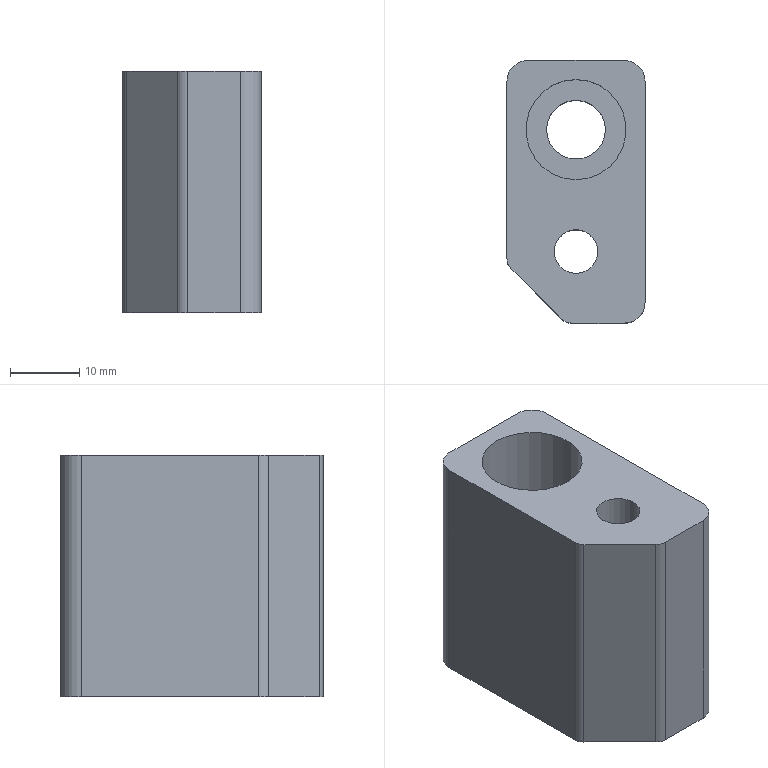Part | NX | features DIE-15 2 | 1 solid | 18 faces | box 20 x 38 x 35 mm | volume 20161 mm3 | plane 9 | cylinder 9 | commonest cylinder face diameters 6 x3 4 x2 6.29 x1 8.29 x1 8.506 x1 14.5 x1
STEP:
#1=CARTESIAN_POINT('',(2411.699,-772.697,858.716));
#2=VERTEX_POINT('',#1);
#3=CARTESIAN_POINT('',(2411.699,-772.697,823.716));
#4=VERTEX_POINT('',#3);
#5=CARTESIAN_POINT('',(2411.699,-772.697,858.716));
#6=DIRECTION('',(0.,0.,-1.));
#7=VECTOR('',#6,1000.);
#8=LINE('',#5,#7);
#9=EDGE_CURVE('',#2,#4,#8,.T.);
#10=ORIENTED_EDGE('',*,*,#9,.F.);
#11=CARTESIAN_POINT('',(2411.699,-804.697,858.716));
#12=VERTEX_POINT('',#11);
#13=CARTESIAN_POINT('',(2411.699,-787.697,858.716));
#14=DIRECTION('',(0.,1.,0.));
#15=VECTOR('',#14,1000.);
#16=LINE('',#13,#15);
#17=EDGE_CURVE('',#12,#2,#16,.T.);
#18=ORIENTED_EDGE('',*,*,#17,.F.);
#19=CARTESIAN_POINT('',(2411.699,-804.697,823.716));
#20=VERTEX_POINT('',#19);
#21=CARTESIAN_POINT('',(2411.699,-804.697,858.716));
#22=DIRECTION('',(0.,0.,-1.));
#23=VECTOR('',#22,1000.);
#24=LINE('',#21,#23);
#25=EDGE_CURVE('',#20,#12,#24,.F.);
#26=ORIENTED_EDGE('',*,*,#25,.F.);
#27=CARTESIAN_POINT('',(2411.699,-787.697,823.716));
#28=DIRECTION('',(0.,-1.,0.));
#29=VECTOR('',#28,1000.);
#30=LINE('',#27,#29);
#31=EDGE_CURVE('',#4,#20,#30,.T.);
#32=ORIENTED_EDGE('',*,*,#31,.F.);
#33=EDGE_LOOP('',(#10,#18,#26,#32));
#34=FACE_BOUND('',#33,.T.);
#35=CARTESIAN_POINT('',(2411.699,-787.697,858.716));
#36=DIRECTION('',(1.,0.,0.));
#37=DIRECTION('',(0.,0.,1.));
#38=AXIS2_PLACEMENT_3D('',#35,#36,#37);
#39=PLANE('',#38);
#40=ADVANCED_FACE('',(#34),#39,.T.);
#41=CARTESIAN_POINT('',(2408.699,-807.697,858.716));
#42=VERTEX_POINT('',#41);
#43=CARTESIAN_POINT('',(2408.699,-807.697,823.716));
#44=VERTEX_POINT('',#43);
#45=CARTESIAN_POINT('',(2408.699,-807.697,858.716));
#46=DIRECTION('',(0.,0.,-1.));
#47=VECTOR('',#46,1000.);
#48=LINE('',#45,#47);
#49=EDGE_CURVE('',#42,#44,#48,.T.);
#50=ORIENTED_EDGE('',*,*,#49,.F.);
#51=CARTESIAN_POINT('',(2401.063,-807.697,858.716));
#52=VERTEX_POINT('',#51);
#53=CARTESIAN_POINT('',(2401.699,-807.697,858.716));
#54=DIRECTION('',(1.,0.,0.));
#55=VECTOR('',#54,1000.);
#56=LINE('',#53,#55);
#57=EDGE_CURVE('',#52,#42,#56,.T.);
#58=ORIENTED_EDGE('',*,*,#57,.F.);
#59=CARTESIAN_POINT('',(2401.063,-807.697,823.716));
#60=VERTEX_POINT('',#59);
#61=CARTESIAN_POINT('',(2401.063,-807.697,858.716));
#62=DIRECTION('',(0.,0.,-1.));
#63=VECTOR('',#62,1000.);
#64=LINE('',#61,#63);
#65=EDGE_CURVE('',#52,#60,#64,.T.);
#66=ORIENTED_EDGE('',*,*,#65,.T.);
#67=CARTESIAN_POINT('',(2401.699,-807.697,823.716));
#68=DIRECTION('',(-1.,0.,0.));
#69=VECTOR('',#68,1000.);
#70=LINE('',#67,#69);
#71=EDGE_CURVE('',#44,#60,#70,.T.);
#72=ORIENTED_EDGE('',*,*,#71,.F.);
#73=EDGE_LOOP('',(#50,#58,#66,#72));
#74=FACE_BOUND('',#73,.T.);
#75=CARTESIAN_POINT('',(2401.699,-807.697,858.716));
#76=DIRECTION('',(0.,-1.,0.));
#77=DIRECTION('',(0.,0.,-1.));
#78=AXIS2_PLACEMENT_3D('',#75,#76,#77);
#79=PLANE('',#78);
#80=ADVANCED_FACE('',(#74),#79,.T.);
#81=CARTESIAN_POINT('',(2391.699,-798.333,823.716));
#82=VERTEX_POINT('',#81);
#83=CARTESIAN_POINT('',(2391.699,-798.333,858.716));
#84=VERTEX_POINT('',#83);
#85=CARTESIAN_POINT('',(2391.699,-798.333,858.716));
#86=DIRECTION('',(0.,0.,1.));
#87=VECTOR('',#86,1000.);
#88=LINE('',#85,#87);
#89=EDGE_CURVE('',#82,#84,#88,.T.);
#90=ORIENTED_EDGE('',*,*,#89,.T.);
#91=CARTESIAN_POINT('',(2391.699,-772.697,858.716));
#92=VERTEX_POINT('',#91);
#93=CARTESIAN_POINT('',(2391.699,-787.697,858.716));
#94=DIRECTION('',(0.,-1.,0.));
#95=VECTOR('',#94,1000.);
#96=LINE('',#93,#95);
#97=EDGE_CURVE('',#92,#84,#96,.T.);
#98=ORIENTED_EDGE('',*,*,#97,.F.);
#99=CARTESIAN_POINT('',(2391.699,-772.697,823.716));
#100=VERTEX_POINT('',#99);
#101=CARTESIAN_POINT('',(2391.699,-772.697,858.716));
#102=DIRECTION('',(0.,0.,-1.));
#103=VECTOR('',#102,1000.);
#104=LINE('',#101,#103);
#105=EDGE_CURVE('',#100,#92,#104,.F.);
#106=ORIENTED_EDGE('',*,*,#105,.F.);
#107=CARTESIAN_POINT('',(2391.699,-787.697,823.716));
#108=DIRECTION('',(0.,1.,0.));
#109=VECTOR('',#108,1000.);
#110=LINE('',#107,#109);
#111=EDGE_CURVE('',#82,#100,#110,.T.);
#112=ORIENTED_EDGE('',*,*,#111,.F.);
#113=EDGE_LOOP('',(#90,#98,#106,#112));
#114=FACE_BOUND('',#113,.T.);
#115=CARTESIAN_POINT('',(2391.699,-787.697,858.716));
#116=DIRECTION('',(-1.,0.,0.));
#117=DIRECTION('',(0.,0.,-1.));
#118=AXIS2_PLACEMENT_3D('',#115,#116,#117);
#119=PLANE('',#118);
#120=ADVANCED_FACE('',(#114),#119,.T.);
#121=CARTESIAN_POINT('',(2394.699,-769.697,858.716));
#122=VERTEX_POINT('',#121);
#123=CARTESIAN_POINT('',(2394.699,-769.697,823.716));
#124=VERTEX_POINT('',#123);
#125=CARTESIAN_POINT('',(2394.699,-769.697,858.716));
#126=DIRECTION('',(0.,0.,-1.));
#127=VECTOR('',#126,1000.);
#128=LINE('',#125,#127);
#129=EDGE_CURVE('',#122,#124,#128,.T.);
#130=ORIENTED_EDGE('',*,*,#129,.F.);
#131=CARTESIAN_POINT('',(2408.699,-769.697,858.716));
#132=VERTEX_POINT('',#131);
#133=CARTESIAN_POINT('',(2401.699,-769.697,858.716));
#134=DIRECTION('',(-1.,0.,0.));
#135=VECTOR('',#134,1000.);
#136=LINE('',#133,#135);
#137=EDGE_CURVE('',#132,#122,#136,.T.);
#138=ORIENTED_EDGE('',*,*,#137,.F.);
#139=CARTESIAN_POINT('',(2408.699,-769.697,823.716));
#140=VERTEX_POINT('',#139);
#141=CARTESIAN_POINT('',(2408.699,-769.697,858.716));
#142=DIRECTION('',(0.,0.,-1.));
#143=VECTOR('',#142,1000.);
#144=LINE('',#141,#143);
#145=EDGE_CURVE('',#140,#132,#144,.F.);
#146=ORIENTED_EDGE('',*,*,#145,.F.);
#147=CARTESIAN_POINT('',(2401.699,-769.697,823.716));
#148=DIRECTION('',(1.,0.,0.));
#149=VECTOR('',#148,1000.);
#150=LINE('',#147,#149);
#151=EDGE_CURVE('',#124,#140,#150,.T.);
#152=ORIENTED_EDGE('',*,*,#151,.F.);
#153=EDGE_LOOP('',(#130,#138,#146,#152));
#154=FACE_BOUND('',#153,.T.);
#155=CARTESIAN_POINT('',(2401.699,-769.697,858.716));
#156=DIRECTION('',(0.,1.,0.));
#157=DIRECTION('',(0.,0.,1.));
#158=AXIS2_PLACEMENT_3D('',#155,#156,#157);
#159=PLANE('',#158);
#160=ADVANCED_FACE('',(#154),#159,.T.);
#161=CARTESIAN_POINT('',(2399.649,-807.111,823.716));
#162=VERTEX_POINT('',#161);
#163=CARTESIAN_POINT('',(2399.649,-807.111,858.716));
#164=VERTEX_POINT('',#163);
#165=CARTESIAN_POINT('',(2399.649,-807.111,858.716));
#166=DIRECTION('',(0.,0.,1.));
#167=VECTOR('',#166,1000.);
#168=LINE('',#165,#167);
#169=EDGE_CURVE('',#162,#164,#168,.T.);
#170=ORIENTED_EDGE('',*,*,#169,.T.);
#171=CARTESIAN_POINT('',(2392.285,-799.747,858.716));
#172=VERTEX_POINT('',#171);
#173=CARTESIAN_POINT('',(2393.467,-800.929,858.716));
#174=DIRECTION('',(0.7071,-0.7071,0.));
#175=VECTOR('',#174,1000.);
#176=LINE('',#173,#175);
#177=EDGE_CURVE('',#164,#172,#176,.F.);
#178=ORIENTED_EDGE('',*,*,#177,.T.);
#179=CARTESIAN_POINT('',(2392.285,-799.747,823.716));
#180=VERTEX_POINT('',#179);
#181=CARTESIAN_POINT('',(2392.285,-799.747,858.716));
#182=DIRECTION('',(0.,0.,-1.));
#183=VECTOR('',#182,1000.);
#184=LINE('',#181,#183);
#185=EDGE_CURVE('',#172,#180,#184,.T.);
#186=ORIENTED_EDGE('',*,*,#185,.T.);
#187=CARTESIAN_POINT('',(2393.467,-800.929,823.716));
#188=DIRECTION('',(-0.7071,0.7071,0.));
#189=VECTOR('',#188,1000.);
#190=LINE('',#187,#189);
#191=EDGE_CURVE('',#180,#162,#190,.F.);
#192=ORIENTED_EDGE('',*,*,#191,.T.);
#193=EDGE_LOOP('',(#170,#178,#186,#192));
#194=FACE_BOUND('',#193,.T.);
#195=CARTESIAN_POINT('',(2393.467,-800.929,858.716));
#196=DIRECTION('',(0.7071,0.7071,0.));
#197=DIRECTION('',(-0.7071,0.7071,0.));
#198=AXIS2_PLACEMENT_3D('',#195,#196,#197);
#199=PLANE('',#198);
#200=ADVANCED_FACE('',(#194),#199,.F.);
#201=ORIENTED_EDGE('',*,*,#105,.T.);
#202=CARTESIAN_POINT('',(2394.699,-772.697,858.716));
#203=DIRECTION('',(0.,0.,-1.));
#204=DIRECTION('',(-1.,0.,0.));
#205=AXIS2_PLACEMENT_3D('',#202,#203,#204);
#206=CIRCLE('',#205,3.);
#207=EDGE_CURVE('',#92,#122,#206,.T.);
#208=ORIENTED_EDGE('',*,*,#207,.T.);
#209=ORIENTED_EDGE('',*,*,#129,.T.);
#210=CARTESIAN_POINT('',(2394.699,-772.697,823.716));
#211=DIRECTION('',(0.,0.,1.));
#212=DIRECTION('',(1.,0.,0.));
#213=AXIS2_PLACEMENT_3D('',#210,#211,#212);
#214=CIRCLE('',#213,3.);
#215=EDGE_CURVE('',#124,#100,#214,.T.);
#216=ORIENTED_EDGE('',*,*,#215,.T.);
#217=EDGE_LOOP('',(#201,#208,#209,#216));
#218=FACE_BOUND('',#217,.T.);
#219=CARTESIAN_POINT('',(2394.699,-772.697,858.716));
#220=DIRECTION('',(0.,0.,-1.));
#221=DIRECTION('',(1.,0.,0.));
#222=AXIS2_PLACEMENT_3D('',#219,#220,#221);
#223=CYLINDRICAL_SURFACE('',#222,3.);
#224=ADVANCED_FACE('',(#218),#223,.T.);
#225=ORIENTED_EDGE('',*,*,#145,.T.);
#226=CARTESIAN_POINT('',(2408.699,-772.697,858.716));
#227=DIRECTION('',(0.,0.,-1.));
#228=DIRECTION('',(-1.,0.,0.));
#229=AXIS2_PLACEMENT_3D('',#226,#227,#228);
#230=CIRCLE('',#229,3.);
#231=EDGE_CURVE('',#132,#2,#230,.T.);
#232=ORIENTED_EDGE('',*,*,#231,.T.);
#233=ORIENTED_EDGE('',*,*,#9,.T.);
#234=CARTESIAN_POINT('',(2408.699,-772.697,823.716));
#235=DIRECTION('',(0.,0.,1.));
#236=DIRECTION('',(1.,0.,0.));
#237=AXIS2_PLACEMENT_3D('',#234,#235,#236);
#238=CIRCLE('',#237,3.);
#239=EDGE_CURVE('',#4,#140,#238,.T.);
#240=ORIENTED_EDGE('',*,*,#239,.T.);
#241=EDGE_LOOP('',(#225,#232,#233,#240));
#242=FACE_BOUND('',#241,.T.);
#243=CARTESIAN_POINT('',(2408.699,-772.697,858.716));
#244=DIRECTION('',(0.,0.,-1.));
#245=DIRECTION('',(1.,0.,0.));
#246=AXIS2_PLACEMENT_3D('',#243,#244,#245);
#247=CYLINDRICAL_SURFACE('',#246,3.);
#248=ADVANCED_FACE('',(#242),#247,.T.);
#249=ORIENTED_EDGE('',*,*,#25,.T.);
#250=CARTESIAN_POINT('',(2408.699,-804.697,858.716));
#251=DIRECTION('',(0.,0.,-1.));
#252=DIRECTION('',(-1.,0.,0.));
#253=AXIS2_PLACEMENT_3D('',#250,#251,#252);
#254=CIRCLE('',#253,3.);
#255=EDGE_CURVE('',#12,#42,#254,.T.);
#256=ORIENTED_EDGE('',*,*,#255,.T.);
#257=ORIENTED_EDGE('',*,*,#49,.T.);
#258=CARTESIAN_POINT('',(2408.699,-804.697,823.716));
#259=DIRECTION('',(0.,0.,1.));
#260=DIRECTION('',(1.,0.,0.));
#261=AXIS2_PLACEMENT_3D('',#258,#259,#260);
#262=CIRCLE('',#261,3.);
#263=EDGE_CURVE('',#44,#20,#262,.T.);
#264=ORIENTED_EDGE('',*,*,#263,.T.);
#265=EDGE_LOOP('',(#249,#256,#257,#264));
#266=FACE_BOUND('',#265,.T.);
#267=CARTESIAN_POINT('',(2408.699,-804.697,858.716));
#268=DIRECTION('',(0.,0.,-1.));
#269=DIRECTION('',(1.,0.,0.));
#270=AXIS2_PLACEMENT_3D('',#267,#268,#269);
#271=CYLINDRICAL_SURFACE('',#270,3.);
#272=ADVANCED_FACE('',(#266),#271,.T.);
#273=CARTESIAN_POINT('',(2401.699,-786.947,847.716));
#274=VERTEX_POINT('',#273);
#275=CARTESIAN_POINT('',(2401.699,-779.697,847.716));
#276=DIRECTION('',(0.,0.,-1.));
#277=DIRECTION('',(0.,-1.,0.));
#278=AXIS2_PLACEMENT_3D('',#275,#276,#277);
#279=CIRCLE('',#278,7.25);
#280=EDGE_CURVE('',#274,#274,#279,.F.);
#281=ORIENTED_EDGE('',*,*,#280,.F.);
#282=EDGE_LOOP('',(#281));
#283=FACE_BOUND('',#282,.T.);
#284=CARTESIAN_POINT('',(2401.699,-786.947,858.716));
#285=VERTEX_POINT('',#284);
#286=CARTESIAN_POINT('',(2401.699,-779.697,858.716));
#287=DIRECTION('',(0.,0.,1.));
#288=DIRECTION('',(0.,-1.,0.));
#289=AXIS2_PLACEMENT_3D('',#286,#287,#288);
#290=CIRCLE('',#289,7.25);
#291=EDGE_CURVE('',#285,#285,#290,.T.);
#292=ORIENTED_EDGE('',*,*,#291,.T.);
#293=EDGE_LOOP('',(#292));
#294=FACE_BOUND('',#293,.T.);
#295=CARTESIAN_POINT('',(2401.699,-779.697,847.716));
#296=DIRECTION('',(0.,0.,1.));
#297=DIRECTION('',(0.,-1.,0.));
#298=AXIS2_PLACEMENT_3D('',#295,#296,#297);
#299=CYLINDRICAL_SURFACE('',#298,7.25);
#300=ADVANCED_FACE('',(#283,#294),#299,.F.);
#301=CARTESIAN_POINT('',(2397.554,-797.347,823.716));
#302=VERTEX_POINT('',#301);
#303=CARTESIAN_POINT('',(2401.699,-797.347,823.716));
#304=DIRECTION('',(0.,0.,-1.));
#305=DIRECTION('',(-1.,0.,0.));
#306=AXIS2_PLACEMENT_3D('',#303,#304,#305);
#307=CIRCLE('',#306,4.145);
#308=EDGE_CURVE('',#302,#302,#307,.F.);
#309=ORIENTED_EDGE('',*,*,#308,.F.);
#310=EDGE_LOOP('',(#309));
#311=FACE_BOUND('',#310,.T.);
#312=CARTESIAN_POINT('',(2405.844,-797.347,853.716));
#313=VERTEX_POINT('',#312);
#314=CARTESIAN_POINT('',(2401.699,-797.347,853.716));
#315=DIRECTION('',(0.,0.,1.));
#316=DIRECTION('',(1.,0.,0.));
#317=AXIS2_PLACEMENT_3D('',#314,#315,#316);
#318=CIRCLE('',#317,4.145);
#319=EDGE_CURVE('',#313,#313,#318,.T.);
#320=ORIENTED_EDGE('',*,*,#319,.T.);
#321=EDGE_LOOP('',(#320));
#322=FACE_BOUND('',#321,.T.);
#323=CARTESIAN_POINT('',(2401.699,-797.347,858.716));
#324=DIRECTION('',(0.,0.,-1.));
#325=DIRECTION('',(1.,0.,0.));
#326=AXIS2_PLACEMENT_3D('',#323,#324,#325);
#327=CYLINDRICAL_SURFACE('',#326,4.145);
#328=ADVANCED_FACE('',(#311,#322),#327,.F.);
#329=ORIENTED_EDGE('',*,*,#185,.F.);
#330=CARTESIAN_POINT('',(2393.699,-798.333,858.716));
#331=DIRECTION('',(0.,0.,1.));
#332=DIRECTION('',(1.,0.,0.));
#333=AXIS2_PLACEMENT_3D('',#330,#331,#332);
#334=CIRCLE('',#333,2.);
#335=EDGE_CURVE('',#84,#172,#334,.T.);
#336=ORIENTED_EDGE('',*,*,#335,.F.);
#337=ORIENTED_EDGE('',*,*,#89,.F.);
#338=CARTESIAN_POINT('',(2393.699,-798.333,823.716));
#339=DIRECTION('',(0.,0.,-1.));
#340=DIRECTION('',(-1.,0.,0.));
#341=AXIS2_PLACEMENT_3D('',#338,#339,#340);
#342=CIRCLE('',#341,2.);
#343=EDGE_CURVE('',#180,#82,#342,.T.);
#344=ORIENTED_EDGE('',*,*,#343,.F.);
#345=EDGE_LOOP('',(#329,#336,#337,#344));
#346=FACE_BOUND('',#345,.T.);
#347=CARTESIAN_POINT('',(2393.699,-798.333,858.716));
#348=DIRECTION('',(0.,0.,1.));
#349=DIRECTION('',(1.,0.,0.));
#350=AXIS2_PLACEMENT_3D('',#347,#348,#349);
#351=CYLINDRICAL_SURFACE('',#350,2.);
#352=ADVANCED_FACE('',(#346),#351,.T.);
#353=ORIENTED_EDGE('',*,*,#65,.F.);
#354=CARTESIAN_POINT('',(2401.063,-805.697,858.716));
#355=DIRECTION('',(0.,0.,1.));
#356=DIRECTION('',(1.,0.,0.));
#357=AXIS2_PLACEMENT_3D('',#354,#355,#356);
#358=CIRCLE('',#357,2.);
#359=EDGE_CURVE('',#164,#52,#358,.T.);
#360=ORIENTED_EDGE('',*,*,#359,.F.);
#361=ORIENTED_EDGE('',*,*,#169,.F.);
#362=CARTESIAN_POINT('',(2401.063,-805.697,823.716));
#363=DIRECTION('',(0.,0.,-1.));
#364=DIRECTION('',(-1.,0.,0.));
#365=AXIS2_PLACEMENT_3D('',#362,#363,#364);
#366=CIRCLE('',#365,2.);
#367=EDGE_CURVE('',#60,#162,#366,.T.);
#368=ORIENTED_EDGE('',*,*,#367,.F.);
#369=EDGE_LOOP('',(#353,#360,#361,#368));
#370=FACE_BOUND('',#369,.T.);
#371=CARTESIAN_POINT('',(2401.063,-805.697,858.716));
#372=DIRECTION('',(0.,0.,-1.));
#373=DIRECTION('',(-1.,0.,0.));
#374=AXIS2_PLACEMENT_3D('',#371,#372,#373);
#375=CYLINDRICAL_SURFACE('',#374,2.);
#376=ADVANCED_FACE('',(#370),#375,.T.);
#377=ORIENTED_EDGE('',*,*,#308,.T.);
#378=EDGE_LOOP('',(#377));
#379=FACE_BOUND('',#378,.T.);
#380=CARTESIAN_POINT('',(2405.952,-779.697,823.716));
#381=VERTEX_POINT('',#380);
#382=CARTESIAN_POINT('',(2401.699,-779.697,823.716));
#383=DIRECTION('',(0.,0.,1.));
#384=DIRECTION('',(1.,0.,0.));
#385=AXIS2_PLACEMENT_3D('',#382,#383,#384);
#386=CIRCLE('',#385,4.253);
#387=EDGE_CURVE('',#381,#381,#386,.T.);
#388=ORIENTED_EDGE('',*,*,#387,.T.);
#389=EDGE_LOOP('',(#388));
#390=FACE_BOUND('',#389,.T.);
#391=ORIENTED_EDGE('',*,*,#191,.F.);
#392=ORIENTED_EDGE('',*,*,#343,.T.);
#393=ORIENTED_EDGE('',*,*,#111,.T.);
#394=ORIENTED_EDGE('',*,*,#215,.F.);
#395=ORIENTED_EDGE('',*,*,#151,.T.);
#396=ORIENTED_EDGE('',*,*,#239,.F.);
#397=ORIENTED_EDGE('',*,*,#31,.T.);
#398=ORIENTED_EDGE('',*,*,#263,.F.);
#399=ORIENTED_EDGE('',*,*,#71,.T.);
#400=ORIENTED_EDGE('',*,*,#367,.T.);
#401=EDGE_LOOP('',(#391,#392,#393,#394,#395,#396,#397,#398,#399,#400));
#402=FACE_BOUND('',#401,.T.);
#403=CARTESIAN_POINT('',(2401.699,-787.697,823.716));
#404=DIRECTION('',(0.,0.,-1.));
#405=DIRECTION('',(0.,1.,0.));
#406=AXIS2_PLACEMENT_3D('',#403,#404,#405);
#407=PLANE('',#406);
#408=ADVANCED_FACE('',(#379,#390,#402),#407,.T.);
#409=CARTESIAN_POINT('',(2405.952,-779.697,847.716));
#410=VERTEX_POINT('',#409);
#411=CARTESIAN_POINT('',(2401.699,-779.697,847.716));
#412=DIRECTION('',(0.,0.,1.));
#413=DIRECTION('',(1.,0.,0.));
#414=AXIS2_PLACEMENT_3D('',#411,#412,#413);
#415=CIRCLE('',#414,4.253);
#416=EDGE_CURVE('',#410,#410,#415,.T.);
#417=ORIENTED_EDGE('',*,*,#416,.F.);
#418=EDGE_LOOP('',(#417));
#419=FACE_BOUND('',#418,.T.);
#420=ORIENTED_EDGE('',*,*,#280,.T.);
#421=EDGE_LOOP('',(#420));
#422=FACE_BOUND('',#421,.T.);
#423=CARTESIAN_POINT('',(2401.699,-779.697,847.716));
#424=DIRECTION('',(0.,0.,-1.));
#425=DIRECTION('',(1.,0.,0.));
#426=AXIS2_PLACEMENT_3D('',#423,#424,#425);
#427=PLANE('',#426);
#428=ADVANCED_FACE('',(#419,#422),#427,.F.);
#429=ORIENTED_EDGE('',*,*,#387,.F.);
#430=EDGE_LOOP('',(#429));
#431=FACE_BOUND('',#430,.T.);
#432=ORIENTED_EDGE('',*,*,#416,.T.);
#433=EDGE_LOOP('',(#432));
#434=FACE_BOUND('',#433,.T.);
#435=CARTESIAN_POINT('',(2401.699,-779.697,822.716));
#436=DIRECTION('',(0.,0.,1.));
#437=DIRECTION('',(0.,-1.,0.));
#438=AXIS2_PLACEMENT_3D('',#435,#436,#437);
#439=CYLINDRICAL_SURFACE('',#438,4.253);
#440=ADVANCED_FACE('',(#431,#434),#439,.F.);
#441=CARTESIAN_POINT('',(2404.844,-797.347,853.716));
#442=VERTEX_POINT('',#441);
#443=CARTESIAN_POINT('',(2401.699,-797.347,853.716));
#444=DIRECTION('',(0.,0.,1.));
#445=DIRECTION('',(1.,0.,0.));
#446=AXIS2_PLACEMENT_3D('',#443,#444,#445);
#447=CIRCLE('',#446,3.145);
#448=EDGE_CURVE('',#442,#442,#447,.F.);
#449=ORIENTED_EDGE('',*,*,#448,.T.);
#450=EDGE_LOOP('',(#449));
#451=FACE_BOUND('',#450,.T.);
#452=CARTESIAN_POINT('',(2404.844,-797.347,858.716));
#453=VERTEX_POINT('',#452);
#454=CARTESIAN_POINT('',(2401.699,-797.347,858.716));
#455=DIRECTION('',(0.,0.,1.));
#456=DIRECTION('',(1.,0.,0.));
#457=AXIS2_PLACEMENT_3D('',#454,#455,#456);
#458=CIRCLE('',#457,3.145);
#459=EDGE_CURVE('',#453,#453,#458,.F.);
#460=ORIENTED_EDGE('',*,*,#459,.F.);
#461=EDGE_LOOP('',(#460));
#462=FACE_BOUND('',#461,.T.);
#463=CARTESIAN_POINT('',(2401.699,-797.347,858.716));
#464=DIRECTION('',(0.,0.,-1.));
#465=DIRECTION('',(1.,0.,0.));
#466=AXIS2_PLACEMENT_3D('',#463,#464,#465);
#467=CYLINDRICAL_SURFACE('',#466,3.145);
#468=ADVANCED_FACE('',(#451,#462),#467,.F.);
#469=ORIENTED_EDGE('',*,*,#459,.T.);
#470=EDGE_LOOP('',(#469));
#471=FACE_BOUND('',#470,.T.);
#472=ORIENTED_EDGE('',*,*,#291,.F.);
#473=EDGE_LOOP('',(#472));
#474=FACE_BOUND('',#473,.T.);
#475=ORIENTED_EDGE('',*,*,#97,.T.);
#476=ORIENTED_EDGE('',*,*,#335,.T.);
#477=ORIENTED_EDGE('',*,*,#177,.F.);
#478=ORIENTED_EDGE('',*,*,#359,.T.);
#479=ORIENTED_EDGE('',*,*,#57,.T.);
#480=ORIENTED_EDGE('',*,*,#255,.F.);
#481=ORIENTED_EDGE('',*,*,#17,.T.);
#482=ORIENTED_EDGE('',*,*,#231,.F.);
#483=ORIENTED_EDGE('',*,*,#137,.T.);
#484=ORIENTED_EDGE('',*,*,#207,.F.);
#485=EDGE_LOOP('',(#475,#476,#477,#478,#479,#480,#481,#482,#483,#484));
#486=FACE_BOUND('',#485,.T.);
#487=CARTESIAN_POINT('',(2401.699,-787.697,858.716));
#488=DIRECTION('',(0.,0.,1.));
#489=DIRECTION('',(0.,-1.,0.));
#490=AXIS2_PLACEMENT_3D('',#487,#488,#489);
#491=PLANE('',#490);
#492=ADVANCED_FACE('',(#471,#474,#486),#491,.T.);
#493=ORIENTED_EDGE('',*,*,#319,.F.);
#494=EDGE_LOOP('',(#493));
#495=FACE_BOUND('',#494,.T.);
#496=ORIENTED_EDGE('',*,*,#448,.F.);
#497=EDGE_LOOP('',(#496));
#498=FACE_BOUND('',#497,.T.);
#499=CARTESIAN_POINT('',(2401.699,-788.697,853.716));
#500=DIRECTION('',(0.,0.,1.));
#501=DIRECTION('',(1.,0.,0.));
#502=AXIS2_PLACEMENT_3D('',#499,#500,#501);
#503=PLANE('',#502);
#504=ADVANCED_FACE('',(#495,#498),#503,.F.);
#505=CLOSED_SHELL('',(#40,#80,#120,#160,#200,#224,#248,#272,#300,#328,#352,#376,#408,#428,#440,#468,#492,#504));
#506=MANIFOLD_SOLID_BREP('',#505);
#507=(LENGTH_UNIT()NAMED_UNIT(*)SI_UNIT(.MILLI.,.METRE.));
#508=UNCERTAINTY_MEASURE_WITH_UNIT(LENGTH_MEASURE(0.00001),#507,'','');
#509=(NAMED_UNIT(*)PLANE_ANGLE_UNIT()SI_UNIT($,.RADIAN.));
#510=(NAMED_UNIT(*)SI_UNIT($,.STERADIAN.)SOLID_ANGLE_UNIT());
#511=(GEOMETRIC_REPRESENTATION_CONTEXT(3)GLOBAL_UNCERTAINTY_ASSIGNED_CONTEXT((#508))GLOBAL_UNIT_ASSIGNED_CONTEXT((#507,#509,#510))REPRESENTATION_CONTEXT('',''));
#512=ADVANCED_BREP_SHAPE_REPRESENTATION('',(#506),#511);